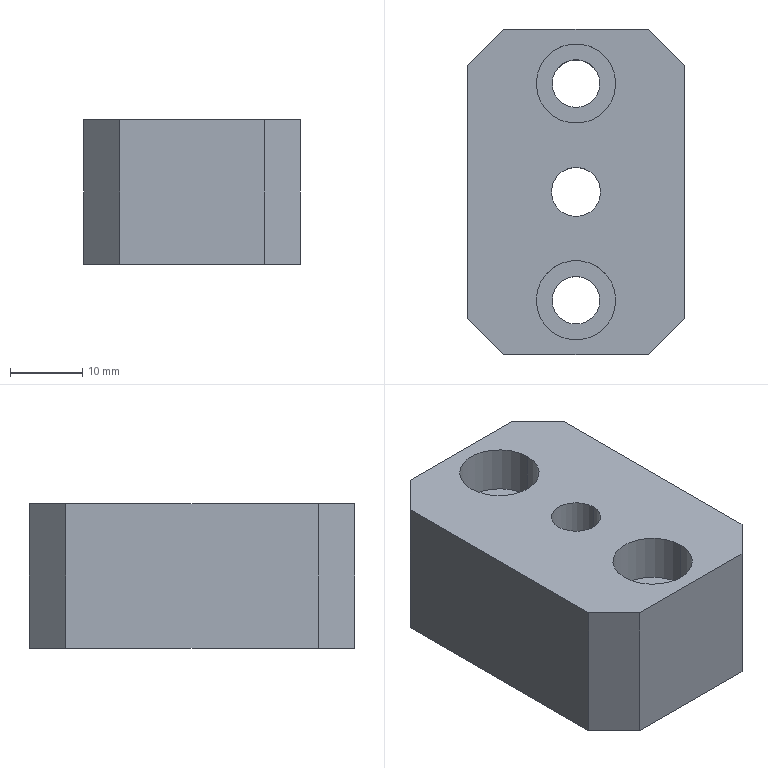Part | STEP file | 0217_206_Base | 1 solid | 22 faces | box 30 x 45 x 20 mm | volume 23102 mm3 | plane 12 | cylinder 10 | commonest cylinder face diameters 6.6 x4 11 x4 6.8 x2